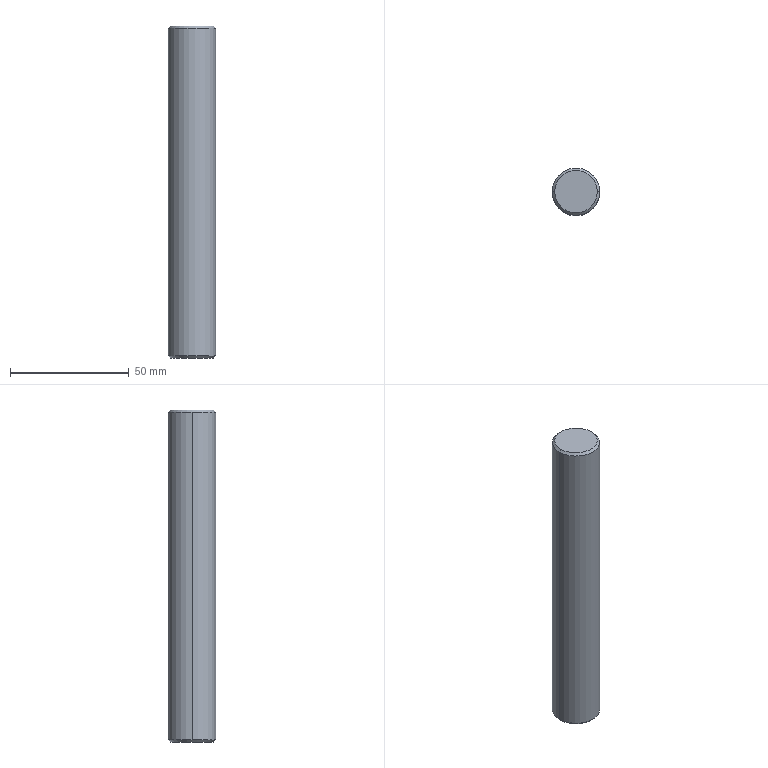Part | SolidWorks | features Chamfer 1, Extrusion 1 | 1 solid | 8 faces | box 20 x 20 x 140 mm | volume 43922 mm3 | cone 4 | cylinder 2 | plane 2 | commonest cylinder face diameters 20 x2
STEP:
#1=CARTESIAN_POINT('',(9.,0.,0.));
#2=VERTEX_POINT('',#1);
#3=CARTESIAN_POINT('',(-9.,0.,0.));
#4=VERTEX_POINT('',#3);
#5=CARTESIAN_POINT('',(0.,0.,0.));
#6=DIRECTION('',(0.,0.,1.));
#7=DIRECTION('',(1.,0.,0.));
#8=AXIS2_PLACEMENT_3D('',#5,#6,#7);
#9=CIRCLE('',#8,9.);
#10=EDGE_CURVE('',#2,#4,#9,.T.);
#11=ORIENTED_EDGE('',*,*,#10,.F.);
#12=CARTESIAN_POINT('',(10.,0.,-1.));
#13=VERTEX_POINT('',#12);
#14=CARTESIAN_POINT('',(9.,0.,0.));
#15=DIRECTION('',(0.7071,0.,-0.7071));
#16=VECTOR('',#15,1000.);
#17=LINE('',#14,#16);
#18=EDGE_CURVE('',#2,#13,#17,.T.);
#19=ORIENTED_EDGE('',*,*,#18,.T.);
#20=CARTESIAN_POINT('',(-10.,0.,-1.));
#21=VERTEX_POINT('',#20);
#22=CARTESIAN_POINT('',(0.,0.,-1.));
#23=DIRECTION('',(0.,0.,-1.));
#24=DIRECTION('',(1.,0.,0.));
#25=AXIS2_PLACEMENT_3D('',#22,#23,#24);
#26=CIRCLE('',#25,10.);
#27=EDGE_CURVE('',#21,#13,#26,.T.);
#28=ORIENTED_EDGE('',*,*,#27,.F.);
#29=CARTESIAN_POINT('',(-9.,0.,0.));
#30=DIRECTION('',(-0.7071,0.,-0.7071));
#31=VECTOR('',#30,1000.);
#32=LINE('',#29,#31);
#33=EDGE_CURVE('',#4,#21,#32,.T.);
#34=ORIENTED_EDGE('',*,*,#33,.F.);
#35=EDGE_LOOP('',(#11,#19,#28,#34));
#36=FACE_OUTER_BOUND('',#35,.T.);
#37=CARTESIAN_POINT('',(0.,0.,0.));
#38=DIRECTION('',(0.,0.,-1.));
#39=DIRECTION('',(-1.,0.,0.));
#40=AXIS2_PLACEMENT_3D('',#37,#38,#39);
#41=CONICAL_SURFACE('',#40,9.,0.7854);
#42=ADVANCED_FACE('',(#36),#41,.T.);
#43=CARTESIAN_POINT('',(-9.,0.,-140.));
#44=VERTEX_POINT('',#43);
#45=CARTESIAN_POINT('',(9.,0.,-140.));
#46=VERTEX_POINT('',#45);
#47=CARTESIAN_POINT('',(0.,0.,-140.));
#48=DIRECTION('',(0.,0.,-1.));
#49=DIRECTION('',(1.,0.,0.));
#50=AXIS2_PLACEMENT_3D('',#47,#48,#49);
#51=CIRCLE('',#50,9.);
#52=EDGE_CURVE('',#44,#46,#51,.T.);
#53=ORIENTED_EDGE('',*,*,#52,.F.);
#54=CARTESIAN_POINT('',(-10.,0.,-139.));
#55=VERTEX_POINT('',#54);
#56=CARTESIAN_POINT('',(-10.,0.,-139.));
#57=DIRECTION('',(-0.7071,0.,0.7071));
#58=VECTOR('',#57,1000.);
#59=LINE('',#56,#58);
#60=EDGE_CURVE('',#44,#55,#59,.T.);
#61=ORIENTED_EDGE('',*,*,#60,.T.);
#62=CARTESIAN_POINT('',(10.,0.,-139.));
#63=VERTEX_POINT('',#62);
#64=CARTESIAN_POINT('',(0.,0.,-139.));
#65=DIRECTION('',(0.,0.,1.));
#66=DIRECTION('',(1.,0.,0.));
#67=AXIS2_PLACEMENT_3D('',#64,#65,#66);
#68=CIRCLE('',#67,10.);
#69=EDGE_CURVE('',#63,#55,#68,.T.);
#70=ORIENTED_EDGE('',*,*,#69,.F.);
#71=CARTESIAN_POINT('',(10.,0.,-139.));
#72=DIRECTION('',(0.7071,0.,0.7071));
#73=VECTOR('',#72,1000.);
#74=LINE('',#71,#73);
#75=EDGE_CURVE('',#46,#63,#74,.T.);
#76=ORIENTED_EDGE('',*,*,#75,.F.);
#77=EDGE_LOOP('',(#53,#61,#70,#76));
#78=FACE_OUTER_BOUND('',#77,.T.);
#79=CARTESIAN_POINT('',(0.,0.,-139.));
#80=DIRECTION('',(0.,0.,1.));
#81=DIRECTION('',(1.,0.,0.));
#82=AXIS2_PLACEMENT_3D('',#79,#80,#81);
#83=CONICAL_SURFACE('',#82,10.,0.7854);
#84=ADVANCED_FACE('',(#78),#83,.T.);
#85=ORIENTED_EDGE('',*,*,#69,.T.);
#86=CARTESIAN_POINT('',(-10.,0.,-140.));
#87=DIRECTION('',(0.,0.,1.));
#88=VECTOR('',#87,1000.);
#89=LINE('',#86,#88);
#90=EDGE_CURVE('',#55,#21,#89,.T.);
#91=ORIENTED_EDGE('',*,*,#90,.T.);
#92=ORIENTED_EDGE('',*,*,#27,.T.);
#93=CARTESIAN_POINT('',(10.,0.,-140.));
#94=DIRECTION('',(0.,0.,1.));
#95=VECTOR('',#94,1000.);
#96=LINE('',#93,#95);
#97=EDGE_CURVE('',#63,#13,#96,.T.);
#98=ORIENTED_EDGE('',*,*,#97,.F.);
#99=EDGE_LOOP('',(#85,#91,#92,#98));
#100=FACE_OUTER_BOUND('',#99,.T.);
#101=CARTESIAN_POINT('',(0.,0.,-140.));
#102=DIRECTION('',(0.,0.,1.));
#103=DIRECTION('',(1.,0.,0.));
#104=AXIS2_PLACEMENT_3D('',#101,#102,#103);
#105=CYLINDRICAL_SURFACE('',#104,10.);
#106=ADVANCED_FACE('',(#100),#105,.T.);
#107=ORIENTED_EDGE('',*,*,#90,.F.);
#108=CARTESIAN_POINT('',(0.,0.,-139.));
#109=DIRECTION('',(0.,0.,1.));
#110=DIRECTION('',(1.,0.,0.));
#111=AXIS2_PLACEMENT_3D('',#108,#109,#110);
#112=CIRCLE('',#111,10.);
#113=EDGE_CURVE('',#55,#63,#112,.T.);
#114=ORIENTED_EDGE('',*,*,#113,.T.);
#115=ORIENTED_EDGE('',*,*,#97,.T.);
#116=CARTESIAN_POINT('',(0.,0.,-1.));
#117=DIRECTION('',(0.,0.,-1.));
#118=DIRECTION('',(1.,0.,0.));
#119=AXIS2_PLACEMENT_3D('',#116,#117,#118);
#120=CIRCLE('',#119,10.);
#121=EDGE_CURVE('',#13,#21,#120,.T.);
#122=ORIENTED_EDGE('',*,*,#121,.T.);
#123=EDGE_LOOP('',(#107,#114,#115,#122));
#124=FACE_OUTER_BOUND('',#123,.T.);
#125=CARTESIAN_POINT('',(0.,0.,-140.));
#126=DIRECTION('',(0.,0.,1.));
#127=DIRECTION('',(1.,0.,0.));
#128=AXIS2_PLACEMENT_3D('',#125,#126,#127);
#129=CYLINDRICAL_SURFACE('',#128,10.);
#130=ADVANCED_FACE('',(#124),#129,.T.);
#131=CARTESIAN_POINT('',(0.,0.,-140.));
#132=DIRECTION('',(0.,0.,-1.));
#133=DIRECTION('',(1.,0.,0.));
#134=AXIS2_PLACEMENT_3D('',#131,#132,#133);
#135=CIRCLE('',#134,9.);
#136=EDGE_CURVE('',#46,#44,#135,.T.);
#137=ORIENTED_EDGE('',*,*,#136,.T.);
#138=ORIENTED_EDGE('',*,*,#52,.T.);
#139=EDGE_LOOP('',(#137,#138));
#140=FACE_OUTER_BOUND('',#139,.T.);
#141=CARTESIAN_POINT('',(0.,0.,-140.));
#142=DIRECTION('',(0.,0.,1.));
#143=DIRECTION('',(1.,0.,0.));
#144=AXIS2_PLACEMENT_3D('',#141,#142,#143);
#145=PLANE('',#144);
#146=ADVANCED_FACE('',(#140),#145,.F.);
#147=CARTESIAN_POINT('',(0.,0.,0.));
#148=DIRECTION('',(0.,0.,1.));
#149=DIRECTION('',(1.,0.,0.));
#150=AXIS2_PLACEMENT_3D('',#147,#148,#149);
#151=CIRCLE('',#150,9.);
#152=EDGE_CURVE('',#4,#2,#151,.T.);
#153=ORIENTED_EDGE('',*,*,#152,.T.);
#154=ORIENTED_EDGE('',*,*,#10,.T.);
#155=EDGE_LOOP('',(#153,#154));
#156=FACE_OUTER_BOUND('',#155,.T.);
#157=CARTESIAN_POINT('',(0.,0.,0.));
#158=DIRECTION('',(0.,0.,1.));
#159=DIRECTION('',(1.,0.,0.));
#160=AXIS2_PLACEMENT_3D('',#157,#158,#159);
#161=PLANE('',#160);
#162=ADVANCED_FACE('',(#156),#161,.T.);
#163=ORIENTED_EDGE('',*,*,#60,.F.);
#164=ORIENTED_EDGE('',*,*,#136,.F.);
#165=ORIENTED_EDGE('',*,*,#75,.T.);
#166=ORIENTED_EDGE('',*,*,#113,.F.);
#167=EDGE_LOOP('',(#163,#164,#165,#166));
#168=FACE_OUTER_BOUND('',#167,.T.);
#169=CARTESIAN_POINT('',(0.,0.,-139.));
#170=DIRECTION('',(0.,0.,1.));
#171=DIRECTION('',(1.,0.,0.));
#172=AXIS2_PLACEMENT_3D('',#169,#170,#171);
#173=CONICAL_SURFACE('',#172,10.,0.7854);
#174=ADVANCED_FACE('',(#168),#173,.T.);
#175=ORIENTED_EDGE('',*,*,#18,.F.);
#176=ORIENTED_EDGE('',*,*,#152,.F.);
#177=ORIENTED_EDGE('',*,*,#33,.T.);
#178=ORIENTED_EDGE('',*,*,#121,.F.);
#179=EDGE_LOOP('',(#175,#176,#177,#178));
#180=FACE_OUTER_BOUND('',#179,.T.);
#181=CARTESIAN_POINT('',(0.,0.,0.));
#182=DIRECTION('',(0.,0.,-1.));
#183=DIRECTION('',(-1.,0.,0.));
#184=AXIS2_PLACEMENT_3D('',#181,#182,#183);
#185=CONICAL_SURFACE('',#184,9.,0.7854);
#186=ADVANCED_FACE('',(#180),#185,.T.);
#187=CLOSED_SHELL('',(#42,#84,#106,#130,#146,#162,#174,#186));
#188=MANIFOLD_SOLID_BREP('',#187);
#189=CARTESIAN_POINT('',(0.,0.,0.));
#190=DIRECTION('',(0.,0.,1.));
#191=DIRECTION('',(1.,0.,0.));
#192=AXIS2_PLACEMENT_3D('',#189,#190,#191);
#193=(LENGTH_UNIT()NAMED_UNIT(*)SI_UNIT(.MILLI.,.METRE.));
#194=UNCERTAINTY_MEASURE_WITH_UNIT(LENGTH_MEASURE(0.00001),#193,'','');
#195=(NAMED_UNIT(*)PLANE_ANGLE_UNIT()SI_UNIT($,.RADIAN.));
#196=(NAMED_UNIT(*)SI_UNIT($,.STERADIAN.)SOLID_ANGLE_UNIT());
#197=(GEOMETRIC_REPRESENTATION_CONTEXT(3)GLOBAL_UNCERTAINTY_ASSIGNED_CONTEXT((#194))GLOBAL_UNIT_ASSIGNED_CONTEXT((#193,#195,#196))REPRESENTATION_CONTEXT('',''));
#198=ADVANCED_BREP_SHAPE_REPRESENTATION('',(#188,#192),#197);